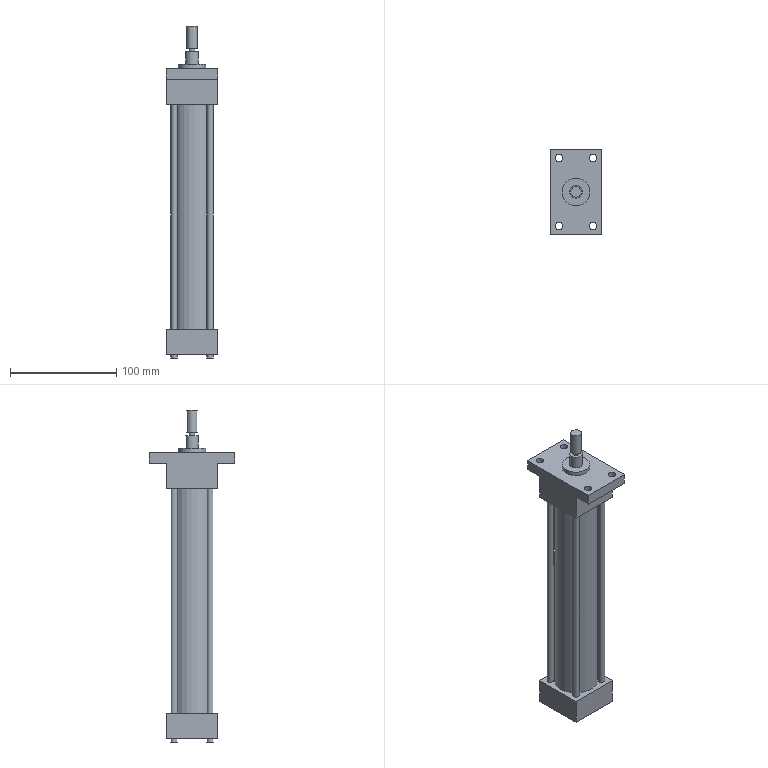Part | NX | features solid 2 | 1 solid | 48 faces | box 48 x 80 x 312 mm | volume 320558 mm3 | plane 28 | cylinder 20 | commonest cylinder face diameters 6 x8 7 x4 10 x3 5 x1 12 x1 26 x1
STEP:
#1=CARTESIAN_POINT('',(-5.,195.,-69.));
#2=VERTEX_POINT('',#1);
#3=CARTESIAN_POINT('',(15.,195.,-69.));
#4=DIRECTION('',(0.,0.,-1.));
#5=DIRECTION('',(-1.,0.,0.));
#6=AXIS2_PLACEMENT_3D('',#3,#4,#5);
#7=CIRCLE('',#6,20.);
#8=EDGE_CURVE('',#2,#2,#7,.T.);
#9=ORIENTED_EDGE('',*,*,#8,.T.);
#10=EDGE_LOOP('',(#9));
#11=FACE_BOUND('',#10,.T.);
#12=CARTESIAN_POINT('',(-5.,195.,-280.));
#13=VERTEX_POINT('',#12);
#14=CARTESIAN_POINT('',(15.,195.,-280.));
#15=DIRECTION('',(0.,0.,-1.));
#16=DIRECTION('',(-1.,0.,0.));
#17=AXIS2_PLACEMENT_3D('',#14,#15,#16);
#18=CIRCLE('',#17,20.);
#19=EDGE_CURVE('',#13,#13,#18,.F.);
#20=ORIENTED_EDGE('',*,*,#19,.T.);
#21=EDGE_LOOP('',(#20));
#22=FACE_BOUND('',#21,.T.);
#23=CARTESIAN_POINT('',(15.,195.,-304.));
#24=DIRECTION('',(0.,0.,1.));
#25=DIRECTION('',(1.,0.,0.));
#26=AXIS2_PLACEMENT_3D('',#23,#24,#25);
#27=CYLINDRICAL_SURFACE('',#26,20.);
#28=ADVANCED_FACE('',(#11,#22),#27,.T.);
#29=CARTESIAN_POINT('',(21.,195.,-19.));
#30=VERTEX_POINT('',#29);
#31=CARTESIAN_POINT('',(15.,195.,-19.));
#32=DIRECTION('',(0.,0.,1.));
#33=DIRECTION('',(1.,0.,0.));
#34=AXIS2_PLACEMENT_3D('',#31,#32,#33);
#35=CIRCLE('',#34,6.);
#36=EDGE_CURVE('',#30,#30,#35,.T.);
#37=ORIENTED_EDGE('',*,*,#36,.T.);
#38=EDGE_LOOP('',(#37));
#39=FACE_BOUND('',#38,.T.);
#40=CARTESIAN_POINT('',(17.5,195.,-19.));
#41=VERTEX_POINT('',#40);
#42=CARTESIAN_POINT('',(15.,195.,-19.));
#43=DIRECTION('',(0.,0.,1.));
#44=DIRECTION('',(1.,0.,0.));
#45=AXIS2_PLACEMENT_3D('',#42,#43,#44);
#46=CIRCLE('',#45,2.5);
#47=EDGE_CURVE('',#41,#41,#46,.T.);
#48=ORIENTED_EDGE('',*,*,#47,.F.);
#49=EDGE_LOOP('',(#48));
#50=FACE_BOUND('',#49,.T.);
#51=CARTESIAN_POINT('',(15.,195.,-19.));
#52=DIRECTION('',(0.,0.,1.));
#53=DIRECTION('',(1.,0.,0.));
#54=AXIS2_PLACEMENT_3D('',#51,#52,#53);
#55=PLANE('',#54);
#56=ADVANCED_FACE('',(#39,#50),#55,.T.);
#57=CARTESIAN_POINT('',(28.,195.,-31.));
#58=VERTEX_POINT('',#57);
#59=CARTESIAN_POINT('',(15.,195.,-31.));
#60=DIRECTION('',(0.,0.,1.));
#61=DIRECTION('',(1.,0.,0.));
#62=AXIS2_PLACEMENT_3D('',#59,#60,#61);
#63=CIRCLE('',#62,13.);
#64=EDGE_CURVE('',#58,#58,#63,.T.);
#65=ORIENTED_EDGE('',*,*,#64,.T.);
#66=EDGE_LOOP('',(#65));
#67=FACE_BOUND('',#66,.T.);
#68=CARTESIAN_POINT('',(21.,195.,-31.));
#69=VERTEX_POINT('',#68);
#70=CARTESIAN_POINT('',(15.,195.,-31.));
#71=DIRECTION('',(0.,0.,1.));
#72=DIRECTION('',(1.,0.,0.));
#73=AXIS2_PLACEMENT_3D('',#70,#71,#72);
#74=CIRCLE('',#73,6.);
#75=EDGE_CURVE('',#69,#69,#74,.F.);
#76=ORIENTED_EDGE('',*,*,#75,.T.);
#77=EDGE_LOOP('',(#76));
#78=FACE_BOUND('',#77,.T.);
#79=CARTESIAN_POINT('',(15.,195.,-31.));
#80=DIRECTION('',(0.,0.,1.));
#81=DIRECTION('',(1.,0.,0.));
#82=AXIS2_PLACEMENT_3D('',#79,#80,#81);
#83=PLANE('',#82);
#84=ADVANCED_FACE('',(#67,#78),#83,.T.);
#85=CARTESIAN_POINT('',(2.5,163.,-35.));
#86=VERTEX_POINT('',#85);
#87=CARTESIAN_POINT('',(-1.,163.,-35.));
#88=DIRECTION('',(0.,0.,1.));
#89=DIRECTION('',(1.,0.,0.));
#90=AXIS2_PLACEMENT_3D('',#87,#88,#89);
#91=CIRCLE('',#90,3.5);
#92=EDGE_CURVE('',#86,#86,#91,.T.);
#93=ORIENTED_EDGE('',*,*,#92,.F.);
#94=EDGE_LOOP('',(#93));
#95=FACE_BOUND('',#94,.T.);
#96=CARTESIAN_POINT('',(34.5,227.,-35.));
#97=VERTEX_POINT('',#96);
#98=CARTESIAN_POINT('',(31.,227.,-35.));
#99=DIRECTION('',(0.,0.,1.));
#100=DIRECTION('',(1.,0.,0.));
#101=AXIS2_PLACEMENT_3D('',#98,#99,#100);
#102=CIRCLE('',#101,3.5);
#103=EDGE_CURVE('',#97,#97,#102,.T.);
#104=ORIENTED_EDGE('',*,*,#103,.F.);
#105=EDGE_LOOP('',(#104));
#106=FACE_BOUND('',#105,.T.);
#107=CARTESIAN_POINT('',(-9.,235.,-35.));
#108=VERTEX_POINT('',#107);
#109=CARTESIAN_POINT('',(39.,235.,-35.));
#110=VERTEX_POINT('',#109);
#111=CARTESIAN_POINT('',(-9.,235.,-35.));
#112=DIRECTION('',(1.,0.,0.));
#113=VECTOR('',#112,1000.);
#114=LINE('',#111,#113);
#115=EDGE_CURVE('',#108,#110,#114,.T.);
#116=ORIENTED_EDGE('',*,*,#115,.F.);
#117=CARTESIAN_POINT('',(-9.,155.,-35.));
#118=VERTEX_POINT('',#117);
#119=CARTESIAN_POINT('',(-9.,219.,-35.));
#120=DIRECTION('',(0.,1.,0.));
#121=VECTOR('',#120,1000.);
#122=LINE('',#119,#121);
#123=EDGE_CURVE('',#118,#108,#122,.T.);
#124=ORIENTED_EDGE('',*,*,#123,.F.);
#125=CARTESIAN_POINT('',(39.,155.,-35.));
#126=VERTEX_POINT('',#125);
#127=CARTESIAN_POINT('',(-9.,155.,-35.));
#128=DIRECTION('',(1.,0.,0.));
#129=VECTOR('',#128,1000.);
#130=LINE('',#127,#129);
#131=EDGE_CURVE('',#118,#126,#130,.T.);
#132=ORIENTED_EDGE('',*,*,#131,.T.);
#133=CARTESIAN_POINT('',(39.,155.,-35.));
#134=DIRECTION('',(0.,1.,0.));
#135=VECTOR('',#134,1000.);
#136=LINE('',#133,#135);
#137=EDGE_CURVE('',#126,#110,#136,.T.);
#138=ORIENTED_EDGE('',*,*,#137,.T.);
#139=EDGE_LOOP('',(#116,#124,#132,#138));
#140=FACE_BOUND('',#139,.T.);
#141=CARTESIAN_POINT('',(2.5,227.,-35.));
#142=VERTEX_POINT('',#141);
#143=CARTESIAN_POINT('',(-1.,227.,-35.));
#144=DIRECTION('',(0.,0.,1.));
#145=DIRECTION('',(1.,0.,0.));
#146=AXIS2_PLACEMENT_3D('',#143,#144,#145);
#147=CIRCLE('',#146,3.5);
#148=EDGE_CURVE('',#142,#142,#147,.T.);
#149=ORIENTED_EDGE('',*,*,#148,.F.);
#150=EDGE_LOOP('',(#149));
#151=FACE_BOUND('',#150,.T.);
#152=CARTESIAN_POINT('',(34.5,163.,-35.));
#153=VERTEX_POINT('',#152);
#154=CARTESIAN_POINT('',(31.,163.,-35.));
#155=DIRECTION('',(0.,0.,1.));
#156=DIRECTION('',(1.,0.,0.));
#157=AXIS2_PLACEMENT_3D('',#154,#155,#156);
#158=CIRCLE('',#157,3.5);
#159=EDGE_CURVE('',#153,#153,#158,.T.);
#160=ORIENTED_EDGE('',*,*,#159,.F.);
#161=EDGE_LOOP('',(#160));
#162=FACE_BOUND('',#161,.T.);
#163=CARTESIAN_POINT('',(2.,195.,-35.));
#164=VERTEX_POINT('',#163);
#165=CARTESIAN_POINT('',(15.,195.,-35.));
#166=DIRECTION('',(0.,0.,-1.));
#167=DIRECTION('',(-1.,0.,0.));
#168=AXIS2_PLACEMENT_3D('',#165,#166,#167);
#169=CIRCLE('',#168,13.);
#170=EDGE_CURVE('',#164,#164,#169,.F.);
#171=ORIENTED_EDGE('',*,*,#170,.F.);
#172=EDGE_LOOP('',(#171));
#173=FACE_BOUND('',#172,.T.);
#174=CARTESIAN_POINT('',(39.,235.,-35.));
#175=DIRECTION('',(0.,0.,-1.));
#176=DIRECTION('',(-1.,0.,0.));
#177=AXIS2_PLACEMENT_3D('',#174,#175,#176);
#178=PLANE('',#177);
#179=ADVANCED_FACE('',(#95,#106,#140,#151,#162,#173),#178,.F.);
#180=CARTESIAN_POINT('',(39.,171.,-45.));
#181=VERTEX_POINT('',#180);
#182=CARTESIAN_POINT('',(-9.,171.,-45.));
#183=VERTEX_POINT('',#182);
#184=CARTESIAN_POINT('',(39.,171.,-45.));
#185=DIRECTION('',(-1.,0.,0.));
#186=VECTOR('',#185,1000.);
#187=LINE('',#184,#186);
#188=EDGE_CURVE('',#181,#183,#187,.T.);
#189=ORIENTED_EDGE('',*,*,#188,.F.);
#190=CARTESIAN_POINT('',(39.,155.,-45.));
#191=VERTEX_POINT('',#190);
#192=CARTESIAN_POINT('',(39.,155.,-45.));
#193=DIRECTION('',(0.,1.,0.));
#194=VECTOR('',#193,1000.);
#195=LINE('',#192,#194);
#196=EDGE_CURVE('',#191,#181,#195,.T.);
#197=ORIENTED_EDGE('',*,*,#196,.F.);
#198=CARTESIAN_POINT('',(-9.,155.,-45.));
#199=VERTEX_POINT('',#198);
#200=CARTESIAN_POINT('',(-9.,155.,-45.));
#201=DIRECTION('',(1.,0.,0.));
#202=VECTOR('',#201,1000.);
#203=LINE('',#200,#202);
#204=EDGE_CURVE('',#199,#191,#203,.T.);
#205=ORIENTED_EDGE('',*,*,#204,.F.);
#206=CARTESIAN_POINT('',(-9.,219.,-45.));
#207=DIRECTION('',(0.,1.,0.));
#208=VECTOR('',#207,1000.);
#209=LINE('',#206,#208);
#210=EDGE_CURVE('',#199,#183,#209,.T.);
#211=ORIENTED_EDGE('',*,*,#210,.T.);
#212=EDGE_LOOP('',(#189,#197,#205,#211));
#213=FACE_BOUND('',#212,.T.);
#214=CARTESIAN_POINT('',(2.5,163.,-45.));
#215=VERTEX_POINT('',#214);
#216=CARTESIAN_POINT('',(-1.,163.,-45.));
#217=DIRECTION('',(0.,0.,1.));
#218=DIRECTION('',(1.,0.,0.));
#219=AXIS2_PLACEMENT_3D('',#216,#217,#218);
#220=CIRCLE('',#219,3.5);
#221=EDGE_CURVE('',#215,#215,#220,.T.);
#222=ORIENTED_EDGE('',*,*,#221,.T.);
#223=EDGE_LOOP('',(#222));
#224=FACE_BOUND('',#223,.T.);
#225=CARTESIAN_POINT('',(34.5,163.,-45.));
#226=VERTEX_POINT('',#225);
#227=CARTESIAN_POINT('',(31.,163.,-45.));
#228=DIRECTION('',(0.,0.,1.));
#229=DIRECTION('',(1.,0.,0.));
#230=AXIS2_PLACEMENT_3D('',#227,#228,#229);
#231=CIRCLE('',#230,3.5);
#232=EDGE_CURVE('',#226,#226,#231,.T.);
#233=ORIENTED_EDGE('',*,*,#232,.T.);
#234=EDGE_LOOP('',(#233));
#235=FACE_BOUND('',#234,.T.);
#236=CARTESIAN_POINT('',(39.,235.,-45.));
#237=DIRECTION('',(0.,0.,-1.));
#238=DIRECTION('',(-1.,0.,0.));
#239=AXIS2_PLACEMENT_3D('',#236,#237,#238);
#240=PLANE('',#239);
#241=ADVANCED_FACE('',(#213,#224,#235),#240,.T.);
#242=ORIENTED_EDGE('',*,*,#115,.T.);
#243=CARTESIAN_POINT('',(39.,235.,-45.));
#244=VERTEX_POINT('',#243);
#245=CARTESIAN_POINT('',(39.,235.,-45.));
#246=DIRECTION('',(0.,0.,1.));
#247=VECTOR('',#246,1000.);
#248=LINE('',#245,#247);
#249=EDGE_CURVE('',#244,#110,#248,.T.);
#250=ORIENTED_EDGE('',*,*,#249,.F.);
#251=CARTESIAN_POINT('',(-9.,235.,-45.));
#252=VERTEX_POINT('',#251);
#253=CARTESIAN_POINT('',(-9.,235.,-45.));
#254=DIRECTION('',(1.,0.,0.));
#255=VECTOR('',#254,1000.);
#256=LINE('',#253,#255);
#257=EDGE_CURVE('',#252,#244,#256,.T.);
#258=ORIENTED_EDGE('',*,*,#257,.F.);
#259=CARTESIAN_POINT('',(-9.,235.,-45.));
#260=DIRECTION('',(0.,0.,1.));
#261=VECTOR('',#260,1000.);
#262=LINE('',#259,#261);
#263=EDGE_CURVE('',#252,#108,#262,.T.);
#264=ORIENTED_EDGE('',*,*,#263,.T.);
#265=EDGE_LOOP('',(#242,#250,#258,#264));
#266=FACE_BOUND('',#265,.T.);
#267=CARTESIAN_POINT('',(-9.,235.,-45.));
#268=DIRECTION('',(0.,-1.,0.));
#269=DIRECTION('',(0.,0.,-1.));
#270=AXIS2_PLACEMENT_3D('',#267,#268,#269);
#271=PLANE('',#270);
#272=ADVANCED_FACE('',(#266),#271,.F.);
#273=CARTESIAN_POINT('',(39.,190.,-57.));
#274=VERTEX_POINT('',#273);
#275=CARTESIAN_POINT('',(39.,195.,-57.));
#276=DIRECTION('',(-1.,0.,0.));
#277=DIRECTION('',(0.,-1.,0.));
#278=AXIS2_PLACEMENT_3D('',#275,#276,#277);
#279=CIRCLE('',#278,5.);
#280=EDGE_CURVE('',#274,#274,#279,.T.);
#281=ORIENTED_EDGE('',*,*,#280,.T.);
#282=EDGE_LOOP('',(#281));
#283=FACE_BOUND('',#282,.T.);
#284=ORIENTED_EDGE('',*,*,#137,.F.);
#285=CARTESIAN_POINT('',(39.,155.,-45.));
#286=DIRECTION('',(0.,0.,1.));
#287=VECTOR('',#286,1000.);
#288=LINE('',#285,#287);
#289=EDGE_CURVE('',#191,#126,#288,.T.);
#290=ORIENTED_EDGE('',*,*,#289,.F.);
#291=ORIENTED_EDGE('',*,*,#196,.T.);
#292=CARTESIAN_POINT('',(39.,171.,-69.));
#293=VERTEX_POINT('',#292);
#294=CARTESIAN_POINT('',(39.,171.,-69.));
#295=DIRECTION('',(0.,0.,1.));
#296=VECTOR('',#295,1000.);
#297=LINE('',#294,#296);
#298=EDGE_CURVE('',#293,#181,#297,.T.);
#299=ORIENTED_EDGE('',*,*,#298,.F.);
#300=CARTESIAN_POINT('',(39.,219.,-69.));
#301=VERTEX_POINT('',#300);
#302=CARTESIAN_POINT('',(39.,219.,-69.));
#303=DIRECTION('',(0.,-1.,0.));
#304=VECTOR('',#303,1000.);
#305=LINE('',#302,#304);
#306=EDGE_CURVE('',#301,#293,#305,.T.);
#307=ORIENTED_EDGE('',*,*,#306,.F.);
#308=CARTESIAN_POINT('',(39.,219.,-45.));
#309=VERTEX_POINT('',#308);
#310=CARTESIAN_POINT('',(39.,219.,-69.));
#311=DIRECTION('',(0.,0.,1.));
#312=VECTOR('',#311,1000.);
#313=LINE('',#310,#312);
#314=EDGE_CURVE('',#301,#309,#313,.T.);
#315=ORIENTED_EDGE('',*,*,#314,.T.);
#316=CARTESIAN_POINT('',(39.,155.,-45.));
#317=DIRECTION('',(0.,1.,0.));
#318=VECTOR('',#317,1000.);
#319=LINE('',#316,#318);
#320=EDGE_CURVE('',#309,#244,#319,.T.);
#321=ORIENTED_EDGE('',*,*,#320,.T.);
#322=ORIENTED_EDGE('',*,*,#249,.T.);
#323=EDGE_LOOP('',(#284,#290,#291,#299,#307,#315,#321,#322));
#324=FACE_BOUND('',#323,.T.);
#325=CARTESIAN_POINT('',(39.,155.,-45.));
#326=DIRECTION('',(1.,0.,0.));
#327=DIRECTION('',(0.,1.,0.));
#328=AXIS2_PLACEMENT_3D('',#325,#326,#327);
#329=PLANE('',#328);
#330=ADVANCED_FACE('',(#283,#324),#329,.T.);
#331=ORIENTED_EDGE('',*,*,#131,.F.);
#332=CARTESIAN_POINT('',(-9.,155.,-45.));
#333=DIRECTION('',(0.,0.,1.));
#334=VECTOR('',#333,1000.);
#335=LINE('',#332,#334);
#336=EDGE_CURVE('',#199,#118,#335,.T.);
#337=ORIENTED_EDGE('',*,*,#336,.F.);
#338=ORIENTED_EDGE('',*,*,#204,.T.);
#339=ORIENTED_EDGE('',*,*,#289,.T.);
#340=EDGE_LOOP('',(#331,#337,#338,#339));
#341=FACE_BOUND('',#340,.T.);
#342=CARTESIAN_POINT('',(-9.,155.,-45.));
#343=DIRECTION('',(0.,-1.,0.));
#344=DIRECTION('',(0.,0.,-1.));
#345=AXIS2_PLACEMENT_3D('',#342,#343,#344);
#346=PLANE('',#345);
#347=ADVANCED_FACE('',(#341),#346,.T.);
#348=CARTESIAN_POINT('',(34.5,227.,-45.));
#349=VERTEX_POINT('',#348);
#350=CARTESIAN_POINT('',(31.,227.,-45.));
#351=DIRECTION('',(0.,0.,1.));
#352=DIRECTION('',(1.,0.,0.));
#353=AXIS2_PLACEMENT_3D('',#350,#351,#352);
#354=CIRCLE('',#353,3.5);
#355=EDGE_CURVE('',#349,#349,#354,.T.);
#356=ORIENTED_EDGE('',*,*,#355,.F.);
#357=EDGE_LOOP('',(#356));
#358=FACE_BOUND('',#357,.T.);
#359=ORIENTED_EDGE('',*,*,#103,.T.);
#360=EDGE_LOOP('',(#359));
#361=FACE_BOUND('',#360,.T.);
#362=CARTESIAN_POINT('',(31.,227.,-45.));
#363=DIRECTION('',(0.,0.,1.));
#364=DIRECTION('',(1.,0.,0.));
#365=AXIS2_PLACEMENT_3D('',#362,#363,#364);
#366=CYLINDRICAL_SURFACE('',#365,3.5);
#367=ADVANCED_FACE('',(#358,#361),#366,.F.);
#368=ORIENTED_EDGE('',*,*,#123,.T.);
#369=ORIENTED_EDGE('',*,*,#263,.F.);
#370=CARTESIAN_POINT('',(-9.,219.,-45.));
#371=VERTEX_POINT('',#370);
#372=CARTESIAN_POINT('',(-9.,219.,-45.));
#373=DIRECTION('',(0.,1.,0.));
#374=VECTOR('',#373,1000.);
#375=LINE('',#372,#374);
#376=EDGE_CURVE('',#371,#252,#375,.T.);
#377=ORIENTED_EDGE('',*,*,#376,.F.);
#378=CARTESIAN_POINT('',(-9.,219.,-69.));
#379=VERTEX_POINT('',#378);
#380=CARTESIAN_POINT('',(-9.,219.,-69.));
#381=DIRECTION('',(0.,0.,1.));
#382=VECTOR('',#381,1000.);
#383=LINE('',#380,#382);
#384=EDGE_CURVE('',#379,#371,#383,.T.);
#385=ORIENTED_EDGE('',*,*,#384,.F.);
#386=CARTESIAN_POINT('',(-9.,171.,-69.));
#387=VERTEX_POINT('',#386);
#388=CARTESIAN_POINT('',(-9.,171.,-69.));
#389=DIRECTION('',(0.,1.,0.));
#390=VECTOR('',#389,1000.);
#391=LINE('',#388,#390);
#392=EDGE_CURVE('',#387,#379,#391,.T.);
#393=ORIENTED_EDGE('',*,*,#392,.F.);
#394=CARTESIAN_POINT('',(-9.,171.,-69.));
#395=DIRECTION('',(0.,0.,1.));
#396=VECTOR('',#395,1000.);
#397=LINE('',#394,#396);
#398=EDGE_CURVE('',#387,#183,#397,.T.);
#399=ORIENTED_EDGE('',*,*,#398,.T.);
#400=ORIENTED_EDGE('',*,*,#210,.F.);
#401=ORIENTED_EDGE('',*,*,#336,.T.);
#402=EDGE_LOOP('',(#368,#369,#377,#385,#393,#399,#400,#401));
#403=FACE_BOUND('',#402,.T.);
#404=CARTESIAN_POINT('',(-9.,219.,-45.));
#405=DIRECTION('',(1.,0.,0.));
#406=DIRECTION('',(0.,0.,-1.));
#407=AXIS2_PLACEMENT_3D('',#404,#405,#406);
#408=PLANE('',#407);
#409=ADVANCED_FACE('',(#403),#408,.F.);
#410=CARTESIAN_POINT('',(2.5,227.,-45.));
#411=VERTEX_POINT('',#410);
#412=CARTESIAN_POINT('',(-1.,227.,-45.));
#413=DIRECTION('',(0.,0.,1.));
#414=DIRECTION('',(1.,0.,0.));
#415=AXIS2_PLACEMENT_3D('',#412,#413,#414);
#416=CIRCLE('',#415,3.5);
#417=EDGE_CURVE('',#411,#411,#416,.T.);
#418=ORIENTED_EDGE('',*,*,#417,.F.);
#419=EDGE_LOOP('',(#418));
#420=FACE_BOUND('',#419,.T.);
#421=ORIENTED_EDGE('',*,*,#148,.T.);
#422=EDGE_LOOP('',(#421));
#423=FACE_BOUND('',#422,.T.);
#424=CARTESIAN_POINT('',(-1.,227.,-45.));
#425=DIRECTION('',(0.,0.,1.));
#426=DIRECTION('',(1.,0.,0.));
#427=AXIS2_PLACEMENT_3D('',#424,#425,#426);
#428=CYLINDRICAL_SURFACE('',#427,3.5);
#429=ADVANCED_FACE('',(#420,#423),#428,.F.);
#430=ORIENTED_EDGE('',*,*,#232,.F.);
#431=EDGE_LOOP('',(#430));
#432=FACE_BOUND('',#431,.T.);
#433=ORIENTED_EDGE('',*,*,#159,.T.);
#434=EDGE_LOOP('',(#433));
#435=FACE_BOUND('',#434,.T.);
#436=CARTESIAN_POINT('',(31.,163.,-45.));
#437=DIRECTION('',(0.,0.,1.));
#438=DIRECTION('',(1.,0.,0.));
#439=AXIS2_PLACEMENT_3D('',#436,#437,#438);
#440=CYLINDRICAL_SURFACE('',#439,3.5);
#441=ADVANCED_FACE('',(#432,#435),#440,.F.);
#442=ORIENTED_EDGE('',*,*,#221,.F.);
#443=EDGE_LOOP('',(#442));
#444=FACE_BOUND('',#443,.T.);
#445=ORIENTED_EDGE('',*,*,#92,.T.);
#446=EDGE_LOOP('',(#445));
#447=FACE_BOUND('',#446,.T.);
#448=CARTESIAN_POINT('',(-1.,163.,-45.));
#449=DIRECTION('',(0.,0.,1.));
#450=DIRECTION('',(1.,0.,0.));
#451=AXIS2_PLACEMENT_3D('',#448,#449,#450);
#452=CYLINDRICAL_SURFACE('',#451,3.5);
#453=ADVANCED_FACE('',(#444,#447),#452,.F.);
#454=CARTESIAN_POINT('',(-9.,219.,-45.));
#455=DIRECTION('',(1.,0.,0.));
#456=VECTOR('',#455,1000.);
#457=LINE('',#454,#456);
#458=EDGE_CURVE('',#371,#309,#457,.T.);
#459=ORIENTED_EDGE('',*,*,#458,.F.);
#460=ORIENTED_EDGE('',*,*,#376,.T.);
#461=ORIENTED_EDGE('',*,*,#257,.T.);
#462=ORIENTED_EDGE('',*,*,#320,.F.);
#463=EDGE_LOOP('',(#459,#460,#461,#462));
#464=FACE_BOUND('',#463,.T.);
#465=ORIENTED_EDGE('',*,*,#417,.T.);
#466=EDGE_LOOP('',(#465));
#467=FACE_BOUND('',#466,.T.);
#468=ORIENTED_EDGE('',*,*,#355,.T.);
#469=EDGE_LOOP('',(#468));
#470=FACE_BOUND('',#469,.T.);
#471=CARTESIAN_POINT('',(39.,235.,-45.));
#472=DIRECTION('',(0.,0.,-1.));
#473=DIRECTION('',(-1.,0.,0.));
#474=AXIS2_PLACEMENT_3D('',#471,#472,#473);
#475=PLANE('',#474);
#476=ADVANCED_FACE('',(#464,#467,#470),#475,.T.);
#477=ORIENTED_EDGE('',*,*,#458,.T.);
#478=ORIENTED_EDGE('',*,*,#314,.F.);
#479=CARTESIAN_POINT('',(-9.,219.,-69.));
#480=DIRECTION('',(1.,0.,0.));
#481=VECTOR('',#480,1000.);
#482=LINE('',#479,#481);
#483=EDGE_CURVE('',#379,#301,#482,.T.);
#484=ORIENTED_EDGE('',*,*,#483,.F.);
#485=ORIENTED_EDGE('',*,*,#384,.T.);
#486=EDGE_LOOP('',(#477,#478,#484,#485));
#487=FACE_BOUND('',#486,.T.);
#488=CARTESIAN_POINT('',(-9.,219.,-69.));
#489=DIRECTION('',(0.,-1.,0.));
#490=DIRECTION('',(0.,0.,-1.));
#491=AXIS2_PLACEMENT_3D('',#488,#489,#490);
#492=PLANE('',#491);
#493=ADVANCED_FACE('',(#487),#492,.F.);
#494=ORIENTED_EDGE('',*,*,#188,.T.);
#495=ORIENTED_EDGE('',*,*,#398,.F.);
#496=CARTESIAN_POINT('',(39.,171.,-69.));
#497=DIRECTION('',(-1.,0.,0.));
#498=VECTOR('',#497,1000.);
#499=LINE('',#496,#498);
#500=EDGE_CURVE('',#293,#387,#499,.T.);
#501=ORIENTED_EDGE('',*,*,#500,.F.);
#502=ORIENTED_EDGE('',*,*,#298,.T.);
#503=EDGE_LOOP('',(#494,#495,#501,#502));
#504=FACE_BOUND('',#503,.T.);
#505=CARTESIAN_POINT('',(39.,171.,-69.));
#506=DIRECTION('',(0.,1.,0.));
#507=DIRECTION('',(0.,0.,1.));
#508=AXIS2_PLACEMENT_3D('',#505,#506,#507);
#509=PLANE('',#508);
#510=ADVANCED_FACE('',(#504),#509,.F.);
#511=CARTESIAN_POINT('',(29.,212.,-69.));
#512=VERTEX_POINT('',#511);
#513=CARTESIAN_POINT('',(32.,212.,-69.));
#514=DIRECTION('',(0.,0.,-1.));
#515=DIRECTION('',(-1.,0.,0.));
#516=AXIS2_PLACEMENT_3D('',#513,#514,#515);
#517=CIRCLE('',#516,3.);
#518=EDGE_CURVE('',#512,#512,#517,.T.);
#519=ORIENTED_EDGE('',*,*,#518,.F.);
#520=EDGE_LOOP('',(#519));
#521=FACE_BOUND('',#520,.T.);
#522=CARTESIAN_POINT('',(-5.,212.,-69.));
#523=VERTEX_POINT('',#522);
#524=CARTESIAN_POINT('',(-2.,212.,-69.));
#525=DIRECTION('',(0.,0.,-1.));
#526=DIRECTION('',(-1.,0.,0.));
#527=AXIS2_PLACEMENT_3D('',#524,#525,#526);
#528=CIRCLE('',#527,3.);
#529=EDGE_CURVE('',#523,#523,#528,.T.);
#530=ORIENTED_EDGE('',*,*,#529,.F.);
#531=EDGE_LOOP('',(#530));
#532=FACE_BOUND('',#531,.T.);
#533=CARTESIAN_POINT('',(-5.,178.,-69.));
#534=VERTEX_POINT('',#533);
#535=CARTESIAN_POINT('',(-2.,178.,-69.));
#536=DIRECTION('',(0.,0.,-1.));
#537=DIRECTION('',(-1.,0.,0.));
#538=AXIS2_PLACEMENT_3D('',#535,#536,#537);
#539=CIRCLE('',#538,3.);
#540=EDGE_CURVE('',#534,#534,#539,.T.);
#541=ORIENTED_EDGE('',*,*,#540,.F.);
#542=EDGE_LOOP('',(#541));
#543=FACE_BOUND('',#542,.T.);
#544=CARTESIAN_POINT('',(29.,178.,-69.));
#545=VERTEX_POINT('',#544);
#546=CARTESIAN_POINT('',(32.,178.,-69.));
#547=DIRECTION('',(0.,0.,-1.));
#548=DIRECTION('',(-1.,0.,0.));
#549=AXIS2_PLACEMENT_3D('',#546,#547,#548);
#550=CIRCLE('',#549,3.);
#551=EDGE_CURVE('',#545,#545,#550,.T.);
#552=ORIENTED_EDGE('',*,*,#551,.F.);
#553=EDGE_LOOP('',(#552));
#554=FACE_BOUND('',#553,.T.);
#555=ORIENTED_EDGE('',*,*,#8,.F.);
#556=EDGE_LOOP('',(#555));
#557=FACE_BOUND('',#556,.T.);
#558=ORIENTED_EDGE('',*,*,#392,.T.);
#559=ORIENTED_EDGE('',*,*,#483,.T.);
#560=ORIENTED_EDGE('',*,*,#306,.T.);
#561=ORIENTED_EDGE('',*,*,#500,.T.);
#562=EDGE_LOOP('',(#558,#559,#560,#561));
#563=FACE_BOUND('',#562,.T.);
#564=CARTESIAN_POINT('',(-9.,219.,-69.));
#565=DIRECTION('',(0.,0.,-1.));
#566=DIRECTION('',(-1.,0.,0.));
#567=AXIS2_PLACEMENT_3D('',#564,#565,#566);
#568=PLANE('',#567);
#569=ADVANCED_FACE('',(#521,#532,#543,#554,#557,#563),#568,.T.);
#570=ORIENTED_EDGE('',*,*,#64,.F.);
#571=EDGE_LOOP('',(#570));
#572=FACE_BOUND('',#571,.T.);
#573=ORIENTED_EDGE('',*,*,#170,.T.);
#574=EDGE_LOOP('',(#573));
#575=FACE_BOUND('',#574,.T.);
#576=CARTESIAN_POINT('',(15.,195.,-31.));
#577=DIRECTION('',(0.,0.,-1.));
#578=DIRECTION('',(-1.,0.,0.));
#579=AXIS2_PLACEMENT_3D('',#576,#577,#578);
#580=CYLINDRICAL_SURFACE('',#579,13.);
#581=ADVANCED_FACE('',(#572,#575),#580,.T.);
#582=ORIENTED_EDGE('',*,*,#75,.F.);
#583=EDGE_LOOP('',(#582));
#584=FACE_BOUND('',#583,.T.);
#585=ORIENTED_EDGE('',*,*,#36,.F.);
#586=EDGE_LOOP('',(#585));
#587=FACE_BOUND('',#586,.T.);
#588=CARTESIAN_POINT('',(15.,195.,-19.));
#589=DIRECTION('',(0.,0.,-1.));
#590=DIRECTION('',(-1.,0.,0.));
#591=AXIS2_PLACEMENT_3D('',#588,#589,#590);
#592=CYLINDRICAL_SURFACE('',#591,6.);
#593=ADVANCED_FACE('',(#584,#587),#592,.T.);
#594=CARTESIAN_POINT('',(-9.,171.,-280.));
#595=VERTEX_POINT('',#594);
#596=CARTESIAN_POINT('',(-9.,219.,-280.));
#597=VERTEX_POINT('',#596);
#598=CARTESIAN_POINT('',(-9.,171.,-280.));
#599=DIRECTION('',(0.,1.,0.));
#600=VECTOR('',#599,1000.);
#601=LINE('',#598,#600);
#602=EDGE_CURVE('',#595,#597,#601,.T.);
#603=ORIENTED_EDGE('',*,*,#602,.T.);
#604=CARTESIAN_POINT('',(-9.,219.,-304.));
#605=VERTEX_POINT('',#604);
#606=CARTESIAN_POINT('',(-9.,219.,-304.));
#607=DIRECTION('',(0.,0.,1.));
#608=VECTOR('',#607,1000.);
#609=LINE('',#606,#608);
#610=EDGE_CURVE('',#605,#597,#609,.T.);
#611=ORIENTED_EDGE('',*,*,#610,.F.);
#612=CARTESIAN_POINT('',(-9.,171.,-304.));
#613=VERTEX_POINT('',#612);
#614=CARTESIAN_POINT('',(-9.,171.,-304.));
#615=DIRECTION('',(0.,1.,0.));
#616=VECTOR('',#615,1000.);
#617=LINE('',#614,#616);
#618=EDGE_CURVE('',#613,#605,#617,.T.);
#619=ORIENTED_EDGE('',*,*,#618,.F.);
#620=CARTESIAN_POINT('',(-9.,171.,-304.));
#621=DIRECTION('',(0.,0.,1.));
#622=VECTOR('',#621,1000.);
#623=LINE('',#620,#622);
#624=EDGE_CURVE('',#613,#595,#623,.T.);
#625=ORIENTED_EDGE('',*,*,#624,.T.);
#626=EDGE_LOOP('',(#603,#611,#619,#625));
#627=FACE_BOUND('',#626,.T.);
#628=CARTESIAN_POINT('',(-9.,171.,-304.));
#629=DIRECTION('',(1.,0.,0.));
#630=DIRECTION('',(0.,0.,-1.));
#631=AXIS2_PLACEMENT_3D('',#628,#629,#630);
#632=PLANE('',#631);
#633=ADVANCED_FACE('',(#627),#632,.F.);
#634=CARTESIAN_POINT('',(39.,219.,-280.));
#635=VERTEX_POINT('',#634);
#636=CARTESIAN_POINT('',(-9.,219.,-280.));
#637=DIRECTION('',(1.,0.,0.));
#638=VECTOR('',#637,1000.);
#639=LINE('',#636,#638);
#640=EDGE_CURVE('',#597,#635,#639,.T.);
#641=ORIENTED_EDGE('',*,*,#640,.T.);
#642=CARTESIAN_POINT('',(39.,219.,-304.));
#643=VERTEX_POINT('',#642);
#644=CARTESIAN_POINT('',(39.,219.,-304.));
#645=DIRECTION('',(0.,0.,1.));
#646=VECTOR('',#645,1000.);
#647=LINE('',#644,#646);
#648=EDGE_CURVE('',#643,#635,#647,.T.);
#649=ORIENTED_EDGE('',*,*,#648,.F.);
#650=CARTESIAN_POINT('',(-9.,219.,-304.));
#651=DIRECTION('',(1.,0.,0.));
#652=VECTOR('',#651,1000.);
#653=LINE('',#650,#652);
#654=EDGE_CURVE('',#605,#643,#653,.T.);
#655=ORIENTED_EDGE('',*,*,#654,.F.);
#656=ORIENTED_EDGE('',*,*,#610,.T.);
#657=EDGE_LOOP('',(#641,#649,#655,#656));
#658=FACE_BOUND('',#657,.T.);
#659=CARTESIAN_POINT('',(-9.,219.,-304.));
#660=DIRECTION('',(0.,-1.,0.));
#661=DIRECTION('',(0.,0.,-1.));
#662=AXIS2_PLACEMENT_3D('',#659,#660,#661);
#663=PLANE('',#662);
#664=ADVANCED_FACE('',(#658),#663,.F.);
#665=CARTESIAN_POINT('',(39.,190.,-292.));
#666=VERTEX_POINT('',#665);
#667=CARTESIAN_POINT('',(39.,195.,-292.));
#668=DIRECTION('',(-1.,0.,0.));
#669=DIRECTION('',(0.,-1.,0.));
#670=AXIS2_PLACEMENT_3D('',#667,#668,#669);
#671=CIRCLE('',#670,5.);
#672=EDGE_CURVE('',#666,#666,#671,.T.);
#673=ORIENTED_EDGE('',*,*,#672,.T.);
#674=EDGE_LOOP('',(#673));
#675=FACE_BOUND('',#674,.T.);
#676=CARTESIAN_POINT('',(39.,171.,-280.));
#677=VERTEX_POINT('',#676);
#678=CARTESIAN_POINT('',(39.,219.,-280.));
#679=DIRECTION('',(0.,-1.,0.));
#680=VECTOR('',#679,1000.);
#681=LINE('',#678,#680);
#682=EDGE_CURVE('',#635,#677,#681,.T.);
#683=ORIENTED_EDGE('',*,*,#682,.T.);
#684=CARTESIAN_POINT('',(39.,171.,-304.));
#685=VERTEX_POINT('',#684);
#686=CARTESIAN_POINT('',(39.,171.,-304.));
#687=DIRECTION('',(0.,0.,1.));
#688=VECTOR('',#687,1000.);
#689=LINE('',#686,#688);
#690=EDGE_CURVE('',#685,#677,#689,.T.);
#691=ORIENTED_EDGE('',*,*,#690,.F.);
#692=CARTESIAN_POINT('',(39.,219.,-304.));
#693=DIRECTION('',(0.,-1.,0.));
#694=VECTOR('',#693,1000.);
#695=LINE('',#692,#694);
#696=EDGE_CURVE('',#643,#685,#695,.T.);
#697=ORIENTED_EDGE('',*,*,#696,.F.);
#698=ORIENTED_EDGE('',*,*,#648,.T.);
#699=EDGE_LOOP('',(#683,#691,#697,#698));
#700=FACE_BOUND('',#699,.T.);
#701=CARTESIAN_POINT('',(39.,219.,-304.));
#702=DIRECTION('',(-1.,0.,0.));
#703=DIRECTION('',(0.,-1.,0.));
#704=AXIS2_PLACEMENT_3D('',#701,#702,#703);
#705=PLANE('',#704);
#706=ADVANCED_FACE('',(#675,#700),#705,.F.);
#707=CARTESIAN_POINT('',(39.,171.,-280.));
#708=DIRECTION('',(-1.,0.,0.));
#709=VECTOR('',#708,1000.);
#710=LINE('',#707,#709);
#711=EDGE_CURVE('',#677,#595,#710,.T.);
#712=ORIENTED_EDGE('',*,*,#711,.T.);
#713=ORIENTED_EDGE('',*,*,#624,.F.);
#714=CARTESIAN_POINT('',(39.,171.,-304.));
#715=DIRECTION('',(-1.,0.,0.));
#716=VECTOR('',#715,1000.);
#717=LINE('',#714,#716);
#718=EDGE_CURVE('',#685,#613,#717,.T.);
#719=ORIENTED_EDGE('',*,*,#718,.F.);
#720=ORIENTED_EDGE('',*,*,#690,.T.);
#721=EDGE_LOOP('',(#712,#713,#719,#720));
#722=FACE_BOUND('',#721,.T.);
#723=CARTESIAN_POINT('',(39.,171.,-304.));
#724=DIRECTION('',(0.,1.,0.));
#725=DIRECTION('',(0.,0.,1.));
#726=AXIS2_PLACEMENT_3D('',#723,#724,#725);
#727=PLANE('',#726);
#728=ADVANCED_FACE('',(#722),#727,.F.);
#729=CARTESIAN_POINT('',(29.,212.,-280.));
#730=VERTEX_POINT('',#729);
#731=CARTESIAN_POINT('',(32.,212.,-280.));
#732=DIRECTION('',(0.,0.,-1.));
#733=DIRECTION('',(-1.,0.,0.));
#734=AXIS2_PLACEMENT_3D('',#731,#732,#733);
#735=CIRCLE('',#734,3.);
#736=EDGE_CURVE('',#730,#730,#735,.T.);
#737=ORIENTED_EDGE('',*,*,#736,.T.);
#738=EDGE_LOOP('',(#737));
#739=FACE_BOUND('',#738,.T.);
#740=CARTESIAN_POINT('',(-5.,212.,-280.));
#741=VERTEX_POINT('',#740);
#742=CARTESIAN_POINT('',(-2.,212.,-280.));
#743=DIRECTION('',(0.,0.,-1.));
#744=DIRECTION('',(-1.,0.,0.));
#745=AXIS2_PLACEMENT_3D('',#742,#743,#744);
#746=CIRCLE('',#745,3.);
#747=EDGE_CURVE('',#741,#741,#746,.T.);
#748=ORIENTED_EDGE('',*,*,#747,.T.);
#749=EDGE_LOOP('',(#748));
#750=FACE_BOUND('',#749,.T.);
#751=CARTESIAN_POINT('',(-5.,178.,-280.));
#752=VERTEX_POINT('',#751);
#753=CARTESIAN_POINT('',(-2.,178.,-280.));
#754=DIRECTION('',(0.,0.,-1.));
#755=DIRECTION('',(-1.,0.,0.));
#756=AXIS2_PLACEMENT_3D('',#753,#754,#755);
#757=CIRCLE('',#756,3.);
#758=EDGE_CURVE('',#752,#752,#757,.T.);
#759=ORIENTED_EDGE('',*,*,#758,.T.);
#760=EDGE_LOOP('',(#759));
#761=FACE_BOUND('',#760,.T.);
#762=CARTESIAN_POINT('',(29.,178.,-280.));
#763=VERTEX_POINT('',#762);
#764=CARTESIAN_POINT('',(32.,178.,-280.));
#765=DIRECTION('',(0.,0.,-1.));
#766=DIRECTION('',(-1.,0.,0.));
#767=AXIS2_PLACEMENT_3D('',#764,#765,#766);
#768=CIRCLE('',#767,3.);
#769=EDGE_CURVE('',#763,#763,#768,.T.);
#770=ORIENTED_EDGE('',*,*,#769,.T.);
#771=EDGE_LOOP('',(#770));
#772=FACE_BOUND('',#771,.T.);
#773=ORIENTED_EDGE('',*,*,#19,.F.);
#774=EDGE_LOOP('',(#773));
#775=FACE_BOUND('',#774,.T.);
#776=ORIENTED_EDGE('',*,*,#602,.F.);
#777=ORIENTED_EDGE('',*,*,#711,.F.);
#778=ORIENTED_EDGE('',*,*,#682,.F.);
#779=ORIENTED_EDGE('',*,*,#640,.F.);
#780=EDGE_LOOP('',(#776,#777,#778,#779));
#781=FACE_BOUND('',#780,.T.);
#782=CARTESIAN_POINT('',(-9.,219.,-280.));
#783=DIRECTION('',(0.,0.,-1.));
#784=DIRECTION('',(-1.,0.,0.));
#785=AXIS2_PLACEMENT_3D('',#782,#783,#784);
#786=PLANE('',#785);
#787=ADVANCED_FACE('',(#739,#750,#761,#772,#775,#781),#786,.F.);
#788=CARTESIAN_POINT('',(35.,212.,-304.));
#789=VERTEX_POINT('',#788);
#790=CARTESIAN_POINT('',(32.,212.,-304.));
#791=DIRECTION('',(0.,0.,1.));
#792=DIRECTION('',(1.,0.,0.));
#793=AXIS2_PLACEMENT_3D('',#790,#791,#792);
#794=CIRCLE('',#793,3.);
#795=EDGE_CURVE('',#789,#789,#794,.T.);
#796=ORIENTED_EDGE('',*,*,#795,.T.);
#797=EDGE_LOOP('',(#796));
#798=FACE_BOUND('',#797,.T.);
#799=CARTESIAN_POINT('',(1.,212.,-304.));
#800=VERTEX_POINT('',#799);
#801=CARTESIAN_POINT('',(-2.,212.,-304.));
#802=DIRECTION('',(0.,0.,1.));
#803=DIRECTION('',(1.,0.,0.));
#804=AXIS2_PLACEMENT_3D('',#801,#802,#803);
#805=CIRCLE('',#804,3.);
#806=EDGE_CURVE('',#800,#800,#805,.T.);
#807=ORIENTED_EDGE('',*,*,#806,.T.);
#808=EDGE_LOOP('',(#807));
#809=FACE_BOUND('',#808,.T.);
#810=CARTESIAN_POINT('',(1.,178.,-304.));
#811=VERTEX_POINT('',#810);
#812=CARTESIAN_POINT('',(-2.,178.,-304.));
#813=DIRECTION('',(0.,0.,1.));
#814=DIRECTION('',(1.,0.,0.));
#815=AXIS2_PLACEMENT_3D('',#812,#813,#814);
#816=CIRCLE('',#815,3.);
#817=EDGE_CURVE('',#811,#811,#816,.T.);
#818=ORIENTED_EDGE('',*,*,#817,.T.);
#819=EDGE_LOOP('',(#818));
#820=FACE_BOUND('',#819,.T.);
#821=CARTESIAN_POINT('',(35.,178.,-304.));
#822=VERTEX_POINT('',#821);
#823=CARTESIAN_POINT('',(32.,178.,-304.));
#824=DIRECTION('',(0.,0.,1.));
#825=DIRECTION('',(1.,0.,0.));
#826=AXIS2_PLACEMENT_3D('',#823,#824,#825);
#827=CIRCLE('',#826,3.);
#828=EDGE_CURVE('',#822,#822,#827,.T.);
#829=ORIENTED_EDGE('',*,*,#828,.T.);
#830=EDGE_LOOP('',(#829));
#831=FACE_BOUND('',#830,.T.);
#832=ORIENTED_EDGE('',*,*,#618,.T.);
#833=ORIENTED_EDGE('',*,*,#654,.T.);
#834=ORIENTED_EDGE('',*,*,#696,.T.);
#835=ORIENTED_EDGE('',*,*,#718,.T.);
#836=EDGE_LOOP('',(#832,#833,#834,#835));
#837=FACE_BOUND('',#836,.T.);
#838=CARTESIAN_POINT('',(15.,195.,-304.));
#839=DIRECTION('',(0.,0.,1.));
#840=DIRECTION('',(1.,0.,0.));
#841=AXIS2_PLACEMENT_3D('',#838,#839,#840);
#842=PLANE('',#841);
#843=ADVANCED_FACE('',(#798,#809,#820,#831,#837),#842,.F.);
#844=CARTESIAN_POINT('',(35.,178.,-307.));
#845=VERTEX_POINT('',#844);
#846=CARTESIAN_POINT('',(32.,178.,-307.));
#847=DIRECTION('',(0.,0.,1.));
#848=DIRECTION('',(1.,0.,0.));
#849=AXIS2_PLACEMENT_3D('',#846,#847,#848);
#850=CIRCLE('',#849,3.);
#851=EDGE_CURVE('',#845,#845,#850,.T.);
#852=ORIENTED_EDGE('',*,*,#851,.F.);
#853=EDGE_LOOP('',(#852));
#854=FACE_BOUND('',#853,.T.);
#855=CARTESIAN_POINT('',(32.,178.,-307.));
#856=DIRECTION('',(0.,0.,1.));
#857=DIRECTION('',(1.,0.,0.));
#858=AXIS2_PLACEMENT_3D('',#855,#856,#857);
#859=PLANE('',#858);
#860=ADVANCED_FACE('',(#854),#859,.F.);
#861=ORIENTED_EDGE('',*,*,#851,.T.);
#862=EDGE_LOOP('',(#861));
#863=FACE_BOUND('',#862,.T.);
#864=ORIENTED_EDGE('',*,*,#828,.F.);
#865=EDGE_LOOP('',(#864));
#866=FACE_BOUND('',#865,.T.);
#867=CARTESIAN_POINT('',(32.,178.,-307.));
#868=DIRECTION('',(0.,0.,1.));
#869=DIRECTION('',(1.,0.,0.));
#870=AXIS2_PLACEMENT_3D('',#867,#868,#869);
#871=CYLINDRICAL_SURFACE('',#870,3.);
#872=ADVANCED_FACE('',(#863,#866),#871,.T.);
#873=ORIENTED_EDGE('',*,*,#551,.T.);
#874=EDGE_LOOP('',(#873));
#875=FACE_BOUND('',#874,.T.);
#876=ORIENTED_EDGE('',*,*,#769,.F.);
#877=EDGE_LOOP('',(#876));
#878=FACE_BOUND('',#877,.T.);
#879=CARTESIAN_POINT('',(32.,178.,-307.));
#880=DIRECTION('',(0.,0.,1.));
#881=DIRECTION('',(1.,0.,0.));
#882=AXIS2_PLACEMENT_3D('',#879,#880,#881);
#883=CYLINDRICAL_SURFACE('',#882,3.);
#884=ADVANCED_FACE('',(#875,#878),#883,.T.);
#885=CARTESIAN_POINT('',(1.,178.,-307.));
#886=VERTEX_POINT('',#885);
#887=CARTESIAN_POINT('',(-2.,178.,-307.));
#888=DIRECTION('',(0.,0.,1.));
#889=DIRECTION('',(1.,0.,0.));
#890=AXIS2_PLACEMENT_3D('',#887,#888,#889);
#891=CIRCLE('',#890,3.);
#892=EDGE_CURVE('',#886,#886,#891,.T.);
#893=ORIENTED_EDGE('',*,*,#892,.F.);
#894=EDGE_LOOP('',(#893));
#895=FACE_BOUND('',#894,.T.);
#896=CARTESIAN_POINT('',(-2.,178.,-307.));
#897=DIRECTION('',(0.,0.,1.));
#898=DIRECTION('',(1.,0.,0.));
#899=AXIS2_PLACEMENT_3D('',#896,#897,#898);
#900=PLANE('',#899);
#901=ADVANCED_FACE('',(#895),#900,.F.);
#902=ORIENTED_EDGE('',*,*,#892,.T.);
#903=EDGE_LOOP('',(#902));
#904=FACE_BOUND('',#903,.T.);
#905=ORIENTED_EDGE('',*,*,#817,.F.);
#906=EDGE_LOOP('',(#905));
#907=FACE_BOUND('',#906,.T.);
#908=CARTESIAN_POINT('',(-2.,178.,-307.));
#909=DIRECTION('',(0.,0.,1.));
#910=DIRECTION('',(1.,0.,0.));
#911=AXIS2_PLACEMENT_3D('',#908,#909,#910);
#912=CYLINDRICAL_SURFACE('',#911,3.);
#913=ADVANCED_FACE('',(#904,#907),#912,.T.);
#914=ORIENTED_EDGE('',*,*,#540,.T.);
#915=EDGE_LOOP('',(#914));
#916=FACE_BOUND('',#915,.T.);
#917=ORIENTED_EDGE('',*,*,#758,.F.);
#918=EDGE_LOOP('',(#917));
#919=FACE_BOUND('',#918,.T.);
#920=CARTESIAN_POINT('',(-2.,178.,-307.));
#921=DIRECTION('',(0.,0.,1.));
#922=DIRECTION('',(1.,0.,0.));
#923=AXIS2_PLACEMENT_3D('',#920,#921,#922);
#924=CYLINDRICAL_SURFACE('',#923,3.);
#925=ADVANCED_FACE('',(#916,#919),#924,.T.);
#926=CARTESIAN_POINT('',(1.,212.,-307.));
#927=VERTEX_POINT('',#926);
#928=CARTESIAN_POINT('',(-2.,212.,-307.));
#929=DIRECTION('',(0.,0.,1.));
#930=DIRECTION('',(1.,0.,0.));
#931=AXIS2_PLACEMENT_3D('',#928,#929,#930);
#932=CIRCLE('',#931,3.);
#933=EDGE_CURVE('',#927,#927,#932,.T.);
#934=ORIENTED_EDGE('',*,*,#933,.F.);
#935=EDGE_LOOP('',(#934));
#936=FACE_BOUND('',#935,.T.);
#937=CARTESIAN_POINT('',(-2.,212.,-307.));
#938=DIRECTION('',(0.,0.,1.));
#939=DIRECTION('',(1.,0.,0.));
#940=AXIS2_PLACEMENT_3D('',#937,#938,#939);
#941=PLANE('',#940);
#942=ADVANCED_FACE('',(#936),#941,.F.);
#943=ORIENTED_EDGE('',*,*,#933,.T.);
#944=EDGE_LOOP('',(#943));
#945=FACE_BOUND('',#944,.T.);
#946=ORIENTED_EDGE('',*,*,#806,.F.);
#947=EDGE_LOOP('',(#946));
#948=FACE_BOUND('',#947,.T.);
#949=CARTESIAN_POINT('',(-2.,212.,-307.));
#950=DIRECTION('',(0.,0.,1.));
#951=DIRECTION('',(1.,0.,0.));
#952=AXIS2_PLACEMENT_3D('',#949,#950,#951);
#953=CYLINDRICAL_SURFACE('',#952,3.);
#954=ADVANCED_FACE('',(#945,#948),#953,.T.);
#955=ORIENTED_EDGE('',*,*,#529,.T.);
#956=EDGE_LOOP('',(#955));
#957=FACE_BOUND('',#956,.T.);
#958=ORIENTED_EDGE('',*,*,#747,.F.);
#959=EDGE_LOOP('',(#958));
#960=FACE_BOUND('',#959,.T.);
#961=CARTESIAN_POINT('',(-2.,212.,-307.));
#962=DIRECTION('',(0.,0.,1.));
#963=DIRECTION('',(1.,0.,0.));
#964=AXIS2_PLACEMENT_3D('',#961,#962,#963);
#965=CYLINDRICAL_SURFACE('',#964,3.);
#966=ADVANCED_FACE('',(#957,#960),#965,.T.);
#967=CARTESIAN_POINT('',(35.,212.,-307.));
#968=VERTEX_POINT('',#967);
#969=CARTESIAN_POINT('',(32.,212.,-307.));
#970=DIRECTION('',(0.,0.,1.));
#971=DIRECTION('',(1.,0.,0.));
#972=AXIS2_PLACEMENT_3D('',#969,#970,#971);
#973=CIRCLE('',#972,3.);
#974=EDGE_CURVE('',#968,#968,#973,.T.);
#975=ORIENTED_EDGE('',*,*,#974,.F.);
#976=EDGE_LOOP('',(#975));
#977=FACE_BOUND('',#976,.T.);
#978=CARTESIAN_POINT('',(32.,212.,-307.));
#979=DIRECTION('',(0.,0.,1.));
#980=DIRECTION('',(1.,0.,0.));
#981=AXIS2_PLACEMENT_3D('',#978,#979,#980);
#982=PLANE('',#981);
#983=ADVANCED_FACE('',(#977),#982,.F.);
#984=ORIENTED_EDGE('',*,*,#974,.T.);
#985=EDGE_LOOP('',(#984));
#986=FACE_BOUND('',#985,.T.);
#987=ORIENTED_EDGE('',*,*,#795,.F.);
#988=EDGE_LOOP('',(#987));
#989=FACE_BOUND('',#988,.T.);
#990=CARTESIAN_POINT('',(32.,212.,-307.));
#991=DIRECTION('',(0.,0.,1.));
#992=DIRECTION('',(1.,0.,0.));
#993=AXIS2_PLACEMENT_3D('',#990,#991,#992);
#994=CYLINDRICAL_SURFACE('',#993,3.);
#995=ADVANCED_FACE('',(#986,#989),#994,.T.);
#996=ORIENTED_EDGE('',*,*,#518,.T.);
#997=EDGE_LOOP('',(#996));
#998=FACE_BOUND('',#997,.T.);
#999=ORIENTED_EDGE('',*,*,#736,.F.);
#1000=EDGE_LOOP('',(#999));
#1001=FACE_BOUND('',#1000,.T.);
#1002=CARTESIAN_POINT('',(32.,212.,-307.));
#1003=DIRECTION('',(0.,0.,1.));
#1004=DIRECTION('',(1.,0.,0.));
#1005=AXIS2_PLACEMENT_3D('',#1002,#1003,#1004);
#1006=CYLINDRICAL_SURFACE('',#1005,3.);
#1007=ADVANCED_FACE('',(#998,#1001),#1006,.T.);
#1008=CARTESIAN_POINT('',(17.5,195.,-16.));
#1009=VERTEX_POINT('',#1008);
#1010=CARTESIAN_POINT('',(15.,195.,-16.));
#1011=DIRECTION('',(0.,0.,1.));
#1012=DIRECTION('',(1.,0.,0.));
#1013=AXIS2_PLACEMENT_3D('',#1010,#1011,#1012);
#1014=CIRCLE('',#1013,2.5);
#1015=EDGE_CURVE('',#1009,#1009,#1014,.T.);
#1016=ORIENTED_EDGE('',*,*,#1015,.T.);
#1017=EDGE_LOOP('',(#1016));
#1018=FACE_BOUND('',#1017,.T.);
#1019=CARTESIAN_POINT('',(20.,195.,-16.));
#1020=VERTEX_POINT('',#1019);
#1021=CARTESIAN_POINT('',(15.,195.,-16.));
#1022=DIRECTION('',(0.,0.,1.));
#1023=DIRECTION('',(1.,0.,0.));
#1024=AXIS2_PLACEMENT_3D('',#1021,#1022,#1023);
#1025=CIRCLE('',#1024,5.);
#1026=EDGE_CURVE('',#1020,#1020,#1025,.T.);
#1027=ORIENTED_EDGE('',*,*,#1026,.F.);
#1028=EDGE_LOOP('',(#1027));
#1029=FACE_BOUND('',#1028,.T.);
#1030=CARTESIAN_POINT('',(15.,195.,-16.));
#1031=DIRECTION('',(0.,0.,1.));
#1032=DIRECTION('',(1.,0.,0.));
#1033=AXIS2_PLACEMENT_3D('',#1030,#1031,#1032);
#1034=PLANE('',#1033);
#1035=ADVANCED_FACE('',(#1018,#1029),#1034,.F.);
#1036=ORIENTED_EDGE('',*,*,#1015,.F.);
#1037=EDGE_LOOP('',(#1036));
#1038=FACE_BOUND('',#1037,.T.);
#1039=ORIENTED_EDGE('',*,*,#47,.T.);
#1040=EDGE_LOOP('',(#1039));
#1041=FACE_BOUND('',#1040,.T.);
#1042=CARTESIAN_POINT('',(15.,195.,-17.5));
#1043=DIRECTION('',(0.,0.,1.));
#1044=DIRECTION('',(1.,0.,0.));
#1045=AXIS2_PLACEMENT_3D('',#1042,#1043,#1044);
#1046=CYLINDRICAL_SURFACE('',#1045,2.5);
#1047=ADVANCED_FACE('',(#1038,#1041),#1046,.T.);
#1048=CARTESIAN_POINT('',(20.,195.,5.));
#1049=VERTEX_POINT('',#1048);
#1050=CARTESIAN_POINT('',(15.,195.,5.));
#1051=DIRECTION('',(0.,0.,1.));
#1052=DIRECTION('',(1.,0.,0.));
#1053=AXIS2_PLACEMENT_3D('',#1050,#1051,#1052);
#1054=CIRCLE('',#1053,5.);
#1055=EDGE_CURVE('',#1049,#1049,#1054,.T.);
#1056=ORIENTED_EDGE('',*,*,#1055,.T.);
#1057=EDGE_LOOP('',(#1056));
#1058=FACE_BOUND('',#1057,.T.);
#1059=CARTESIAN_POINT('',(15.,195.,5.));
#1060=DIRECTION('',(0.,0.,1.));
#1061=DIRECTION('',(1.,0.,0.));
#1062=AXIS2_PLACEMENT_3D('',#1059,#1060,#1061);
#1063=PLANE('',#1062);
#1064=ADVANCED_FACE('',(#1058),#1063,.T.);
#1065=ORIENTED_EDGE('',*,*,#1026,.T.);
#1066=EDGE_LOOP('',(#1065));
#1067=FACE_BOUND('',#1066,.T.);
#1068=ORIENTED_EDGE('',*,*,#1055,.F.);
#1069=EDGE_LOOP('',(#1068));
#1070=FACE_BOUND('',#1069,.T.);
#1071=CARTESIAN_POINT('',(15.,195.,5.));
#1072=DIRECTION('',(0.,0.,-1.));
#1073=DIRECTION('',(-1.,0.,0.));
#1074=AXIS2_PLACEMENT_3D('',#1071,#1072,#1073);
#1075=CYLINDRICAL_SURFACE('',#1074,5.);
#1076=ADVANCED_FACE('',(#1067,#1070),#1075,.T.);
#1077=CARTESIAN_POINT('',(35.,190.,-57.));
#1078=VERTEX_POINT('',#1077);
#1079=CARTESIAN_POINT('',(35.,195.,-57.));
#1080=DIRECTION('',(-1.,0.,0.));
#1081=DIRECTION('',(0.,-1.,0.));
#1082=AXIS2_PLACEMENT_3D('',#1079,#1080,#1081);
#1083=CIRCLE('',#1082,5.);
#1084=EDGE_CURVE('',#1078,#1078,#1083,.T.);
#1085=ORIENTED_EDGE('',*,*,#1084,.F.);
#1086=EDGE_LOOP('',(#1085));
#1087=FACE_BOUND('',#1086,.T.);
#1088=CARTESIAN_POINT('',(35.,195.,-57.));
#1089=DIRECTION('',(-1.,0.,0.));
#1090=DIRECTION('',(0.,-1.,0.));
#1091=AXIS2_PLACEMENT_3D('',#1088,#1089,#1090);
#1092=PLANE('',#1091);
#1093=ADVANCED_FACE('',(#1087),#1092,.F.);
#1094=ORIENTED_EDGE('',*,*,#1084,.T.);
#1095=EDGE_LOOP('',(#1094));
#1096=FACE_BOUND('',#1095,.T.);
#1097=ORIENTED_EDGE('',*,*,#280,.F.);
#1098=EDGE_LOOP('',(#1097));
#1099=FACE_BOUND('',#1098,.T.);
#1100=CARTESIAN_POINT('',(39.,195.,-57.));
#1101=DIRECTION('',(-1.,0.,0.));
#1102=DIRECTION('',(0.,-1.,0.));
#1103=AXIS2_PLACEMENT_3D('',#1100,#1101,#1102);
#1104=CYLINDRICAL_SURFACE('',#1103,5.);
#1105=ADVANCED_FACE('',(#1096,#1099),#1104,.F.);
#1106=CARTESIAN_POINT('',(35.,190.,-292.));
#1107=VERTEX_POINT('',#1106);
#1108=CARTESIAN_POINT('',(35.,195.,-292.));
#1109=DIRECTION('',(-1.,0.,0.));
#1110=DIRECTION('',(0.,-1.,0.));
#1111=AXIS2_PLACEMENT_3D('',#1108,#1109,#1110);
#1112=CIRCLE('',#1111,5.);
#1113=EDGE_CURVE('',#1107,#1107,#1112,.T.);
#1114=ORIENTED_EDGE('',*,*,#1113,.F.);
#1115=EDGE_LOOP('',(#1114));
#1116=FACE_BOUND('',#1115,.T.);
#1117=CARTESIAN_POINT('',(35.,195.,-292.));
#1118=DIRECTION('',(-1.,0.,0.));
#1119=DIRECTION('',(0.,-1.,0.));
#1120=AXIS2_PLACEMENT_3D('',#1117,#1118,#1119);
#1121=PLANE('',#1120);
#1122=ADVANCED_FACE('',(#1116),#1121,.F.);
#1123=ORIENTED_EDGE('',*,*,#1113,.T.);
#1124=EDGE_LOOP('',(#1123));
#1125=FACE_BOUND('',#1124,.T.);
#1126=ORIENTED_EDGE('',*,*,#672,.F.);
#1127=EDGE_LOOP('',(#1126));
#1128=FACE_BOUND('',#1127,.T.);
#1129=CARTESIAN_POINT('',(39.,195.,-292.));
#1130=DIRECTION('',(-1.,0.,0.));
#1131=DIRECTION('',(0.,-1.,0.));
#1132=AXIS2_PLACEMENT_3D('',#1129,#1130,#1131);
#1133=CYLINDRICAL_SURFACE('',#1132,5.);
#1134=ADVANCED_FACE('',(#1125,#1128),#1133,.F.);
#1135=CLOSED_SHELL('',(#28,#56,#84,#179,#241,#272,#330,#347,#367,#409,#429,#441,#453,#476,#493,#510,#569,#581,#593,#633,#664,#706,#728,#787,#843,#860,#872,#884,#901,#913,#925,#942,#954,#966,#983,#995,#1007,#1035,#1047,#1064,#1076,#1093,#1105,#1122,#1134));
#1136=CARTESIAN_POINT('',(28.5,195.,-280.));
#1137=VERTEX_POINT('',#1136);
#1138=CARTESIAN_POINT('',(15.,195.,-280.));
#1139=DIRECTION('',(0.,0.,1.));
#1140=DIRECTION('',(1.,0.,0.));
#1141=AXIS2_PLACEMENT_3D('',#1138,#1139,#1140);
#1142=CIRCLE('',#1141,13.5);
#1143=EDGE_CURVE('',#1137,#1137,#1142,.T.);
#1144=ORIENTED_EDGE('',*,*,#1143,.F.);
#1145=EDGE_LOOP('',(#1144));
#1146=FACE_BOUND('',#1145,.T.);
#1147=CARTESIAN_POINT('',(28.5,195.,-69.));
#1148=VERTEX_POINT('',#1147);
#1149=CARTESIAN_POINT('',(15.,195.,-69.));
#1150=DIRECTION('',(0.,0.,1.));
#1151=DIRECTION('',(1.,0.,0.));
#1152=AXIS2_PLACEMENT_3D('',#1149,#1150,#1151);
#1153=CIRCLE('',#1152,13.5);
#1154=EDGE_CURVE('',#1148,#1148,#1153,.T.);
#1155=ORIENTED_EDGE('',*,*,#1154,.T.);
#1156=EDGE_LOOP('',(#1155));
#1157=FACE_BOUND('',#1156,.T.);
#1158=CARTESIAN_POINT('',(15.,195.,-280.));
#1159=DIRECTION('',(0.,0.,1.));
#1160=DIRECTION('',(1.,0.,0.));
#1161=AXIS2_PLACEMENT_3D('',#1158,#1159,#1160);
#1162=CYLINDRICAL_SURFACE('',#1161,13.5);
#1163=ADVANCED_FACE('',(#1146,#1157),#1162,.F.);
#1164=ORIENTED_EDGE('',*,*,#1143,.T.);
#1165=EDGE_LOOP('',(#1164));
#1166=FACE_BOUND('',#1165,.T.);
#1167=CARTESIAN_POINT('',(15.,195.,-280.));
#1168=DIRECTION('',(0.,0.,1.));
#1169=DIRECTION('',(1.,0.,0.));
#1170=AXIS2_PLACEMENT_3D('',#1167,#1168,#1169);
#1171=PLANE('',#1170);
#1172=ADVANCED_FACE('',(#1166),#1171,.T.);
#1173=ORIENTED_EDGE('',*,*,#1154,.F.);
#1174=EDGE_LOOP('',(#1173));
#1175=FACE_BOUND('',#1174,.T.);
#1176=CARTESIAN_POINT('',(15.,195.,-69.));
#1177=DIRECTION('',(0.,0.,1.));
#1178=DIRECTION('',(1.,0.,0.));
#1179=AXIS2_PLACEMENT_3D('',#1176,#1177,#1178);
#1180=PLANE('',#1179);
#1181=ADVANCED_FACE('',(#1175),#1180,.F.);
#1182=CLOSED_SHELL('',(#1163,#1172,#1181));
#1183=ORIENTED_CLOSED_SHELL('',*,#1182,.F.);
#1184=BREP_WITH_VOIDS('',#1135,(#1183));
#1185=(LENGTH_UNIT()NAMED_UNIT(*)SI_UNIT(.MILLI.,.METRE.));
#1186=UNCERTAINTY_MEASURE_WITH_UNIT(LENGTH_MEASURE(0.00001),#1185,'','');
#1187=(NAMED_UNIT(*)PLANE_ANGLE_UNIT()SI_UNIT($,.RADIAN.));
#1188=(NAMED_UNIT(*)SI_UNIT($,.STERADIAN.)SOLID_ANGLE_UNIT());
#1189=(GEOMETRIC_REPRESENTATION_CONTEXT(3)GLOBAL_UNCERTAINTY_ASSIGNED_CONTEXT((#1186))GLOBAL_UNIT_ASSIGNED_CONTEXT((#1185,#1187,#1188))REPRESENTATION_CONTEXT('',''));
#1190=ADVANCED_BREP_SHAPE_REPRESENTATION('',(#1184),#1189);